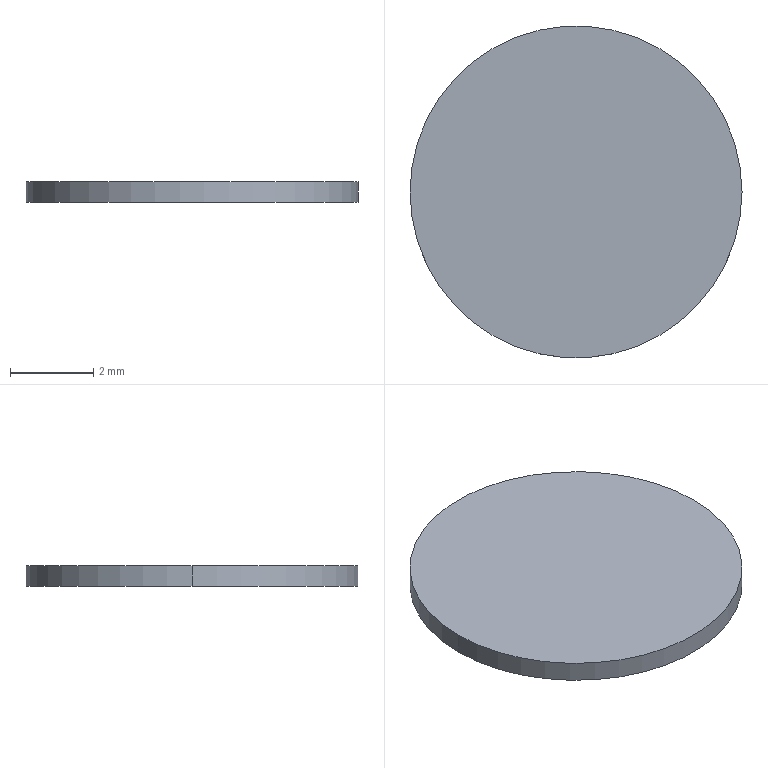Part | Creo | 1 solid | 7 faces | box 8 x 8 x 0.5 mm | volume 23.747 mm3 | cylinder 4 | plane 3 | commonest cylinder face diameters 4.2 x2 8 x2
STEP:
#1=CARTESIAN_POINT('',(0.,0.,0.));
#2=DIRECTION('',(0.,0.,1.));
#3=DIRECTION('',(1.,0.,0.));
#4=AXIS2_PLACEMENT_3D('',#1,#2,#3);
#5=CARTESIAN_POINT('',(-4.,76.272,-9.05));
#6=VERTEX_POINT('',#5);
#7=CARTESIAN_POINT('',(4.,76.272,-9.05));
#8=VERTEX_POINT('',#7);
#9=CARTESIAN_POINT('',(0.,76.272,-9.05));
#10=DIRECTION('',(0.,0.,-1.));
#11=DIRECTION('',(-1.,0.,0.));
#12=AXIS2_PLACEMENT_3D('',#9,#10,#11);
#13=CIRCLE('',#12,4.);
#14=EDGE_CURVE('',#6,#8,#13,.T.);
#15=ORIENTED_EDGE('',*,*,#14,.F.);
#16=CARTESIAN_POINT('',(0.,76.272,-9.05));
#17=DIRECTION('',(0.,0.,-1.));
#18=DIRECTION('',(1.,0.,0.));
#19=AXIS2_PLACEMENT_3D('',#16,#17,#18);
#20=CIRCLE('',#19,4.);
#21=EDGE_CURVE('',#8,#6,#20,.T.);
#22=ORIENTED_EDGE('',*,*,#21,.F.);
#23=EDGE_LOOP('',(#15,#22));
#24=FACE_OUTER_BOUND('',#23,.F.);
#25=CARTESIAN_POINT('',(-2.1,76.272,-9.05));
#26=VERTEX_POINT('',#25);
#27=CARTESIAN_POINT('',(2.1,76.272,-9.05));
#28=VERTEX_POINT('',#27);
#29=CARTESIAN_POINT('',(0.,76.272,-9.05));
#30=DIRECTION('',(0.,0.,-1.));
#31=DIRECTION('',(-1.,0.,0.));
#32=AXIS2_PLACEMENT_3D('',#29,#30,#31);
#33=CIRCLE('',#32,2.1);
#34=EDGE_CURVE('',#26,#28,#33,.T.);
#35=ORIENTED_EDGE('',*,*,#34,.T.);
#36=CARTESIAN_POINT('',(0.,76.272,-9.05));
#37=DIRECTION('',(0.,0.,-1.));
#38=DIRECTION('',(1.,0.,0.));
#39=AXIS2_PLACEMENT_3D('',#36,#37,#38);
#40=CIRCLE('',#39,2.1);
#41=EDGE_CURVE('',#28,#26,#40,.T.);
#42=ORIENTED_EDGE('',*,*,#41,.T.);
#43=EDGE_LOOP('',(#35,#42));
#44=FACE_BOUND('',#43,.F.);
#45=CARTESIAN_POINT('',(0.,0.,-9.05));
#46=DIRECTION('',(0.,0.,-1.));
#47=DIRECTION('',(-1.,0.,0.));
#48=AXIS2_PLACEMENT_3D('',#45,#46,#47);
#49=PLANE('',#48);
#50=ADVANCED_FACE('',(#24,#44),#49,.T.);
#51=ORIENTED_EDGE('',*,*,#14,.T.);
#52=CARTESIAN_POINT('',(4.,76.272,-8.55));
#53=VERTEX_POINT('',#52);
#54=CARTESIAN_POINT('',(4.,76.272,-9.05));
#55=DIRECTION('',(0.,0.,1.));
#56=VECTOR('',#55,0.5);
#57=LINE('',#54,#56);
#58=EDGE_CURVE('',#8,#53,#57,.T.);
#59=ORIENTED_EDGE('',*,*,#58,.T.);
#60=CARTESIAN_POINT('',(-4.,76.272,-8.55));
#61=VERTEX_POINT('',#60);
#62=CARTESIAN_POINT('',(0.,76.272,-8.55));
#63=DIRECTION('',(0.,0.,-1.));
#64=DIRECTION('',(-1.,0.,0.));
#65=AXIS2_PLACEMENT_3D('',#62,#63,#64);
#66=CIRCLE('',#65,4.);
#67=EDGE_CURVE('',#61,#53,#66,.T.);
#68=ORIENTED_EDGE('',*,*,#67,.F.);
#69=CARTESIAN_POINT('',(-4.,76.272,-9.05));
#70=DIRECTION('',(0.,0.,1.));
#71=VECTOR('',#70,0.5);
#72=LINE('',#69,#71);
#73=EDGE_CURVE('',#6,#61,#72,.T.);
#74=ORIENTED_EDGE('',*,*,#73,.F.);
#75=EDGE_LOOP('',(#51,#59,#68,#74));
#76=FACE_OUTER_BOUND('',#75,.F.);
#77=CARTESIAN_POINT('',(0.,76.272,-9.05));
#78=DIRECTION('',(0.,0.,-1.));
#79=DIRECTION('',(-1.,0.,0.));
#80=AXIS2_PLACEMENT_3D('',#77,#78,#79);
#81=CYLINDRICAL_SURFACE('',#80,4.);
#82=ADVANCED_FACE('',(#76),#81,.T.);
#83=ORIENTED_EDGE('',*,*,#21,.T.);
#84=ORIENTED_EDGE('',*,*,#73,.T.);
#85=CARTESIAN_POINT('',(0.,76.272,-8.55));
#86=DIRECTION('',(0.,0.,-1.));
#87=DIRECTION('',(1.,0.,0.));
#88=AXIS2_PLACEMENT_3D('',#85,#86,#87);
#89=CIRCLE('',#88,4.);
#90=EDGE_CURVE('',#53,#61,#89,.T.);
#91=ORIENTED_EDGE('',*,*,#90,.F.);
#92=ORIENTED_EDGE('',*,*,#58,.F.);
#93=EDGE_LOOP('',(#83,#84,#91,#92));
#94=FACE_OUTER_BOUND('',#93,.F.);
#95=CARTESIAN_POINT('',(0.,76.272,-9.05));
#96=DIRECTION('',(0.,0.,-1.));
#97=DIRECTION('',(-1.,0.,0.));
#98=AXIS2_PLACEMENT_3D('',#95,#96,#97);
#99=CYLINDRICAL_SURFACE('',#98,4.);
#100=ADVANCED_FACE('',(#94),#99,.T.);
#101=ORIENTED_EDGE('',*,*,#67,.T.);
#102=ORIENTED_EDGE('',*,*,#90,.T.);
#103=EDGE_LOOP('',(#101,#102));
#104=FACE_OUTER_BOUND('',#103,.F.);
#105=CARTESIAN_POINT('',(0.,0.,-8.55));
#106=DIRECTION('',(0.,0.,-1.));
#107=DIRECTION('',(-1.,0.,0.));
#108=AXIS2_PLACEMENT_3D('',#105,#106,#107);
#109=PLANE('',#108);
#110=ADVANCED_FACE('',(#104),#109,.F.);
#111=ORIENTED_EDGE('',*,*,#34,.F.);
#112=CARTESIAN_POINT('',(-2.1,76.272,-8.95));
#113=VERTEX_POINT('',#112);
#114=CARTESIAN_POINT('',(-2.1,76.272,-9.05));
#115=DIRECTION('',(0.,0.,1.));
#116=VECTOR('',#115,0.1);
#117=LINE('',#114,#116);
#118=EDGE_CURVE('',#26,#113,#117,.T.);
#119=ORIENTED_EDGE('',*,*,#118,.T.);
#120=CARTESIAN_POINT('',(2.1,76.272,-8.95));
#121=VERTEX_POINT('',#120);
#122=CARTESIAN_POINT('',(0.,76.272,-8.95));
#123=DIRECTION('',(0.,0.,1.));
#124=DIRECTION('',(1.,0.,0.));
#125=AXIS2_PLACEMENT_3D('',#122,#123,#124);
#126=CIRCLE('',#125,2.1);
#127=EDGE_CURVE('',#121,#113,#126,.T.);
#128=ORIENTED_EDGE('',*,*,#127,.F.);
#129=CARTESIAN_POINT('',(2.1,76.272,-9.05));
#130=DIRECTION('',(0.,0.,1.));
#131=VECTOR('',#130,0.1);
#132=LINE('',#129,#131);
#133=EDGE_CURVE('',#28,#121,#132,.T.);
#134=ORIENTED_EDGE('',*,*,#133,.F.);
#135=EDGE_LOOP('',(#111,#119,#128,#134));
#136=FACE_OUTER_BOUND('',#135,.F.);
#137=CARTESIAN_POINT('',(0.,76.272,-9.05));
#138=DIRECTION('',(0.,0.,-1.));
#139=DIRECTION('',(-1.,0.,0.));
#140=AXIS2_PLACEMENT_3D('',#137,#138,#139);
#141=CYLINDRICAL_SURFACE('',#140,2.1);
#142=ADVANCED_FACE('',(#136),#141,.F.);
#143=ORIENTED_EDGE('',*,*,#41,.F.);
#144=ORIENTED_EDGE('',*,*,#133,.T.);
#145=CARTESIAN_POINT('',(0.,76.272,-8.95));
#146=DIRECTION('',(0.,0.,1.));
#147=DIRECTION('',(-1.,0.,0.));
#148=AXIS2_PLACEMENT_3D('',#145,#146,#147);
#149=CIRCLE('',#148,2.1);
#150=EDGE_CURVE('',#113,#121,#149,.T.);
#151=ORIENTED_EDGE('',*,*,#150,.F.);
#152=ORIENTED_EDGE('',*,*,#118,.F.);
#153=EDGE_LOOP('',(#143,#144,#151,#152));
#154=FACE_OUTER_BOUND('',#153,.F.);
#155=CARTESIAN_POINT('',(0.,76.272,-9.05));
#156=DIRECTION('',(0.,0.,-1.));
#157=DIRECTION('',(-1.,0.,0.));
#158=AXIS2_PLACEMENT_3D('',#155,#156,#157);
#159=CYLINDRICAL_SURFACE('',#158,2.1);
#160=ADVANCED_FACE('',(#154),#159,.F.);
#161=ORIENTED_EDGE('',*,*,#127,.T.);
#162=ORIENTED_EDGE('',*,*,#150,.T.);
#163=EDGE_LOOP('',(#161,#162));
#164=FACE_OUTER_BOUND('',#163,.F.);
#165=CARTESIAN_POINT('',(0.,0.,-8.95));
#166=DIRECTION('',(0.,0.,-1.));
#167=DIRECTION('',(-1.,0.,0.));
#168=AXIS2_PLACEMENT_3D('',#165,#166,#167);
#169=PLANE('',#168);
#170=ADVANCED_FACE('',(#164),#169,.T.);
#171=CLOSED_SHELL('',(#50,#82,#100,#110,#142,#160,#170));
#172=MANIFOLD_SOLID_BREP('',#171);
#173=(LENGTH_UNIT()NAMED_UNIT(*)SI_UNIT(.MILLI.,.METRE.));
#174=UNCERTAINTY_MEASURE_WITH_UNIT(LENGTH_MEASURE(0.001132),#173,'','');
#175=(NAMED_UNIT(*)PLANE_ANGLE_UNIT()SI_UNIT($,.RADIAN.));
#176=PLANE_ANGLE_MEASURE_WITH_UNIT(PLANE_ANGLE_MEASURE(0.01745),#175);
#177=(CONVERSION_BASED_UNIT('DEGREE',#176)NAMED_UNIT(*)PLANE_ANGLE_UNIT());
#178=(NAMED_UNIT(*)SI_UNIT($,.STERADIAN.)SOLID_ANGLE_UNIT());
#179=(GEOMETRIC_REPRESENTATION_CONTEXT(3)GLOBAL_UNCERTAINTY_ASSIGNED_CONTEXT((#174))GLOBAL_UNIT_ASSIGNED_CONTEXT((#173,#177,#178))REPRESENTATION_CONTEXT('',''));
#180=ADVANCED_BREP_SHAPE_REPRESENTATION('',(#4,#172),#179);